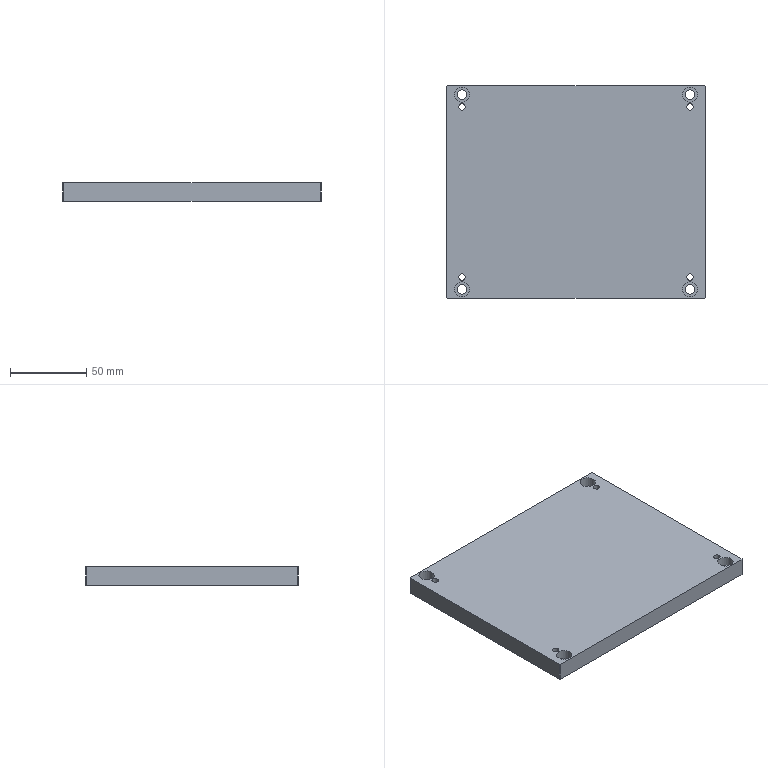Part | STEP file | 1 solid | 26 faces | box 170 x 140 x 12 mm | volume 282154 mm3 | plane 14 | cylinder 12 | commonest cylinder face diameters 4.2 x4 6.5 x4 10 x4